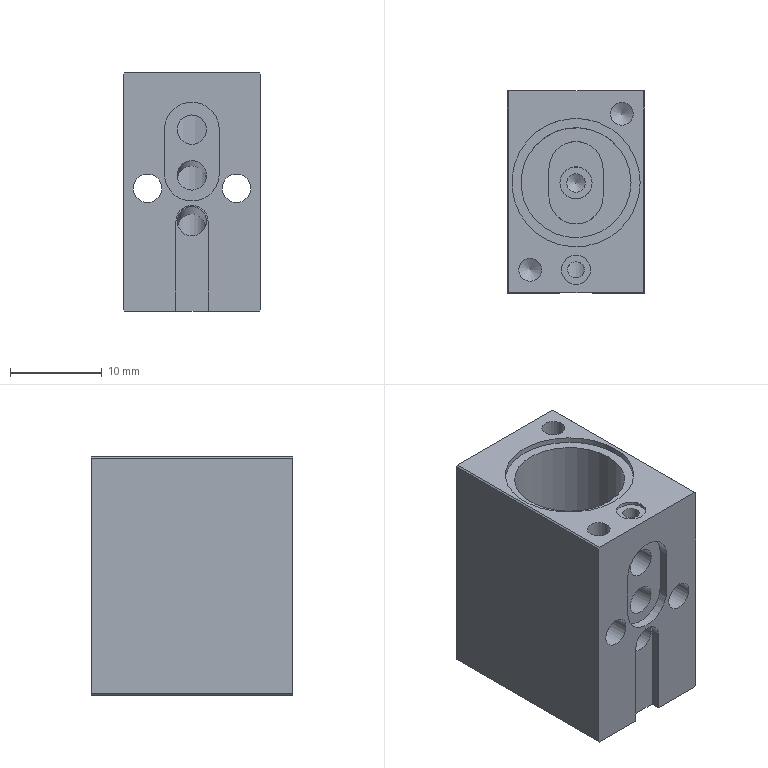NC program | NX | posted with a generic post | part box 15 x 22 x 26 mm
Whole program:
N10 G17 G21 G94 G90
(DRILLING_1 , TOOL : D3开粗)
N12 T14 M6
N14 G54
N16 G17 G0 G90 X-0.015 Y14.756 B0. C0. S3000 M3
N18 G43 Z3.431 H14
N20 G94 G81 G99 Z-0.569 F100. R3.431
N22 G80
(DRILLING_1_COPY , TOOL : D3开粗)
N24 G0 X-0.015 Y9.775
N26 G43 Z2.995 H14
N28 G81 Z-1.005 F100. R2.995
N30 G80
N32 M5
(DRILLING_1_COPY_1 , TOOL : D3点钻)
N34 T06 M6
N36 G54
N38 G17 G43 G0 G90 X-0.015 Y14.756 B0. C0. S3000 H6 M3
N40 Z3.431
N42 G94 G81 G99 Z-1.069 F200. R3.431
N44 G80
(DRILLING_1_COPY_COPY , TOOL : D3点钻)
N46 G0 X-0.015 Y9.775
N48 G43 Z2.995 H6
N50 G81 Z-1.505 F200. R2.995
N52 G80
N54 M5
(DRILLING_1_COPY_1_COPY , TOOL : D3.2钻头)
N56 T04 M6
N58 G54
N60 G17 G43 G0 G90 X-0.015 Y14.756 B0. C0. S3000 H4 M3
N62 Z3.431
N64 G94 G81 G99 Z-8.569 F200. R3.431
N66 G80
(DRILLING_1_COPY_COPY_COPY , TOOL : D3.2钻头)
N68 G0 X-0.015 Y9.775
N70 G43 Z2.995 H4
N72 G81 Z-12.005 F200. R2.995
N74 G80
N76 M5
(3_AXIS_DEBURRING , TOOL : R0.5)
N78 T18 M6
N80 G54
N82 G17 G43 G0 G90 X-0.959 Y9.797 B0. C0. S3000 H18 M3
N84 Z13.779
N86 Z0.214
N88 G94 G1 X-0.974 Y9.796 Z0.119 F243.
N90 X-1.013 Y9.793 Z0.028
N92 X-1.134 Y9.783 Z-0.131
N94 X-1.185 Y9.756 Z-0.19
N96 X-1.221 Y9.696 Z-0.245
N98 X-1.243 Y9.618 Z-0.292
N100 X-1.25 Y9.535 Z-0.325
N102 Y9.449 Z-0.352 F270.
N104 Y9.361 Z-0.38
N106 X-1.234 Y9.275 Z-0.408
N108 X-1.198 Y9.194 Z-0.416
N110 X-1.163 Y9.113 Z-0.424
N112 X-1.111 Y9.041 Z-0.431
N114 X-1.06 Y8.969 Z-0.438
N116 X-1.009 Y8.897 Z-0.445
N118 X-0.945 Y8.836 Z-0.451
N120 X-0.88 Y8.776 Z-0.457
N122 X-0.816 Y8.716 Z-0.463
N124 X-0.741 Y8.669 Z-0.467
N126 X-0.666 Y8.623 Z-0.472
N128 X-0.59 Y8.577 Z-0.476
N130 X-0.508 Y8.547 Z-0.479
N132 X-0.425 Y8.517 Z-0.483
N134 X-0.342 Y8.486 Z-0.486
N136 X-0.255 Y8.47 Z-0.484
N138 X-0.169 Y8.454 Z-0.483
N140 X-0.082 Y8.438 Z-0.482
N142 X-0.017 Y8.437 Z-0.478
N144 X0.047 Y8.435 Z-0.474
N146 X0.112 Y8.434 Z-0.47
N148 X0.176 Y8.432 Z-0.466
N150 X0.179
N152 X0.267 Y8.464 Z-0.471
N154 X0.352 Y8.495 Z-0.476
N156 X0.438 Y8.526 Z-0.482
N158 X0.517 Y8.564 Z-0.478
N160 X0.597 Y8.602 Z-0.474
N162 X0.676 Y8.641 Z-0.47
N164 X0.746 Y8.694 Z-0.465
N166 X0.816 Y8.748 Z-0.46
N168 X0.886 Y8.801 Z-0.454
N170 X0.944 Y8.868 Z-0.448
N172 X1.003 Y8.934 Z-0.441
N174 X1.061 Y9.001 Z-0.435
N176 X1.107 Y9.077 Z-0.425
N178 X1.152 Y9.153 Z-0.415
N180 X1.198 Y9.229 Z-0.405
N182 X1.222 Y9.314 Z-0.394
N184 Y9.404 Z-0.357
N186 Y9.49 Z-0.322
N188 X1.215 Y9.572 Z-0.281
N190 X1.194 Y9.649 Z-0.228
N192 X1.158 Y9.707 Z-0.168
N194 X1.107 Y9.734 Z-0.105
N196 X0.989 Y9.747 Z0.056
N198 X0.951 Y9.752 Z0.148
N200 X0.936 Y9.753 Z0.243
N202 X0.912 Y9.754 Z0.405
N204 X0.888 Y9.75 Z0.571
N206 X0.863 Y9.741 Z0.741
N208 X0.838 Y9.73 Z0.915
N210 X0.812 Y9.715 Z1.092
N212 X0.786 Y9.697 Z1.271
N214 X0.76 Y9.676 Z1.454
N216 X0.733 Y9.654 Z1.638
N218 X0.706 Y9.629 Z1.824
N220 X0.679 Y9.604 Z2.012
N222 X0.652 Y9.577 Z2.201
N224 X0.625 Y9.55 Z2.39
N226 X0.598 Y9.522 Z2.58
N228 X0.57 Y9.494 Z2.769
N230 X0.543 Y9.468 Z2.958
N232 X0.516 Y9.441 Z3.146
N234 X0.489 Y9.417 Z3.333
N236 X0.463 Y9.393 Z3.518
N238 X0.436 Y9.372 Z3.701
N240 X0.41 Y9.353 Z3.882
N242 X0.384 Y9.337 Z4.06
N244 X0.359 Y9.324 Z4.234
N246 X0.334 Y9.315 Z4.405
N248 X0.309 Y9.31 Z4.573
N250 X0.285 Y9.308 Z4.736
N252 X0.261 Y9.312 Z4.894
N254 X0.238 Y9.32 Z5.047
N256 X0.216 Y9.334 Z5.195
N258 X0.194 Y9.354 Z5.337
N260 X0.173 Y9.38 Z5.473
N262 X0.153 Y9.412 Z5.602
N264 X0.134 Y9.452 Z5.724
N266 X0.116 Y9.498 Z5.839
N268 X0.098 Y9.553 Z5.946
N270 X0.081 Y9.615 Z6.045
N272 X0.066 Y9.686 Z6.136
N274 X0.051 Y9.765 Z6.218
N276 X0.038 Y9.854 Z6.29
N278 X0.028 Y9.928 Z6.339
N280 X0.019 Y10.009 Z6.385
N282 X0.01 Y10.097 Z6.429
N284 X0.001 Y10.192 Z6.47
N286 X-0.008 Y10.294 Z6.509
N288 X-0.016 Y10.401 Z6.545
N290 X-0.024 Y10.514 Z6.578
N292 X-0.032 Y10.633 Z6.609
N294 X-0.04 Y10.756 Z6.637
N296 X-0.047 Y10.883 Z6.662
N298 X-0.054 Y11.014 Z6.685
N300 X-0.061 Y11.148 Z6.705
N302 X-0.067 Y11.285 Z6.723
N304 X-0.074 Y11.425 Z6.738
N306 X-0.079 Y11.567 Z6.75
N308 X-0.085 Y11.71 Z6.76
N310 X-0.09 Y11.855 Z6.767
N312 X-0.095 Y12. Z6.771
N314 X-0.099 Y12.145 Z6.773
N316 X-0.103 Y12.291 Z6.772
N318 X-0.107 Y12.435 Z6.768
N320 X-0.11 Y12.579 Z6.762
N322 X-0.113 Y12.721 Z6.753
N324 X-0.116 Y12.862 Z6.741
N326 X-0.118 Y13. Z6.727
N328 X-0.12 Y13.135 Z6.71
N330 X-0.121 Y13.267 Z6.69
N332 X-0.122 Y13.395 Z6.668
N334 Y13.519 Z6.642
N336 Y13.639 Z6.615
N338 Y13.754 Z6.584
N340 X-0.121 Y13.863 Z6.551
N342 X-0.119 Y13.966 Z6.515
N344 X-0.117 Y14.063 Z6.476
N346 X-0.115 Y14.154 Z6.434
N348 X-0.112 Y14.237 Z6.39
N350 X-0.108 Y14.312 Z6.343
N352 X-0.104 Y14.38 Z6.293
N354 X-0.098 Y14.458 Z6.222
N356 X-0.09 Y14.526 Z6.142
N358 X-0.081 Y14.584 Z6.054
N360 X-0.071 Y14.635 Z5.957
N362 X-0.06 Y14.676 Z5.853
N364 X-0.047 Y14.71 Z5.742
N366 X-0.033 Y14.736 Z5.623
N368 X-0.019 Y14.755 Z5.498
N370 X-0.003 Y14.767 Z5.366
N372 X0.014 Y14.772 Z5.229
N374 X0.031 Y14.771 Z5.086
N376 X0.05 Y14.765 Z4.938
N378 X0.069 Y14.754 Z4.785
N380 X0.088 Y14.737 Z4.627
N382 X0.109 Y14.717 Z4.466
N384 X0.13 Y14.692 Z4.3
N386 X0.151 Y14.663 Z4.132
N388 X0.173 Y14.631 Z3.96
N390 X0.196 Y14.597 Z3.786
N392 X0.219 Y14.559 Z3.609
N394 X0.242 Y14.52 Z3.431
N396 X0.265 Y14.479 Z3.25
N398 X0.289 Y14.437 Z3.069
N400 X0.312 Y14.393 Z2.887
N402 X0.336 Y14.35 Z2.704
N404 X0.36 Y14.306 Z2.521
N406 X0.383 Y14.262 Z2.339
N408 X0.407 Y14.219 Z2.157
N410 X0.43 Y14.177 Z1.976
N412 X0.454 Y14.136 Z1.796
N414 X0.477 Y14.098 Z1.618
N416 X0.499 Y14.061 Z1.443
N418 X0.522 Y14.028 Z1.269
N420 X0.544 Y13.997 Z1.098
N422 X0.565 Y13.969 Z0.931
N424 X0.586 Y13.946 Z0.767
N426 X0.606 Y13.926 Z0.606
N428 X0.625 Y13.912 Z0.45
N430 X0.638 Y13.904 Z0.354 F243.
N432 X0.669 Y13.883 Z0.262
N434 X0.769 Y13.819 Z0.101
N436 X0.825 Y13.812 Z0.052
N438 X0.896 Y13.839 Z0.019
N440 X0.969 Y13.888 Z0.001
N442 X1.03 Y13.945 Z-0.001
N444 X1.062 Y13.981 Z0.003 F270.
N446 X1.105 Y14.058 Z0.01
N448 X1.149 Y14.135 Z0.017
N450 X1.193 Y14.213 Z0.025
N452 X1.22 Y14.297 Z0.033
N454 X1.247 Y14.382 Z0.041
N456 X1.275 Y14.466 Z0.049
N458 X1.284 Y14.555 Z0.057
N460 X1.292 Y14.643 Z0.064
N462 X1.301 Y14.732 Z0.072
N464 X1.294 Y14.82 Z0.081
N466 X1.286 Y14.909 Z0.09
N468 X1.279 Y14.997 Z0.1
N470 X1.253 Y15.083 Z0.108
N472 X1.227 Y15.168 Z0.116
N474 X1.201 Y15.254 Z0.124
N476 X1.158 Y15.332 Z0.132
N478 X1.115 Y15.41 Z0.139
N480 X1.072 Y15.489 Z0.147
N482 X1.014 Y15.557 Z0.154
N484 X0.957 Y15.625 Z0.16
N486 X0.899 Y15.694 Z0.167
N488 X0.828 Y15.749 Z0.172
N490 X0.758 Y15.804 Z0.177
N492 X0.687 Y15.859 Z0.182
N494 X0.607 Y15.899 Z0.186
N496 X0.526 Y15.939 Z0.19
N498 X0.446 Y15.978 Z0.194
N500 X0.361 Y16.002 Z0.197
N502 X0.276 Y16.026 Z0.201
N504 X0.191 Y16.05 Z0.205
N506 X0.112 Y16.058 Z0.21
N508 X0.033 Y16.066 Z0.215
N510 X-0.046 Y16.074 Z0.221
N512 X-0.125 Y16.082 Z0.226
N514 X-0.207 Y16.06 Z0.217
N516 X-0.289 Y16.037 Z0.208
N518 X-0.37 Y16.014 Z0.198
N520 X-0.49 Y15.967 Z0.193
N522 X-0.609 Y15.921 Z0.188
N524 X-0.664 Y15.886 Z0.185
N526 X-0.718 Y15.851 Z0.182
N528 X-0.773 Y15.817 Z0.178
N530 X-0.828 Y15.782 Z0.175
N532 X-0.892 Y15.72 Z0.169
N534 X-0.957 Y15.658 Z0.163
N536 X-1.021 Y15.596 Z0.157
N538 X-1.072 Y15.522 Z0.15
N540 X-1.122 Y15.448 Z0.143
N542 X-1.173 Y15.374 Z0.136
N544 X-1.208 Y15.292 Z0.128
N546 X-1.242 Y15.21 Z0.12
N548 X-1.277 Y15.127 Z0.112
N550 X-1.294 Y15.04 Z0.104
N552 X-1.311 Y14.952 Z0.095
N554 X-1.328 Y14.865 Z0.087
N556 X-1.327 Y14.776 Z0.078
N558 X-1.326 Y14.687 Z0.07
N560 X-1.325 Y14.598 Z0.061
N562 X-1.309 Y14.51 Z0.055
N564 X-1.292 Y14.423 Z0.048
N566 X-1.276 Y14.335 Z0.042
N568 X-1.24 Y14.254 Z0.034
N570 X-1.203 Y14.172 Z0.025
N572 X-1.167 Y14.091 Z0.017
N574 X-1.116 Y14.019 Z0.01
N576 X-1.064 Y13.946 Z0.003
N578 X-1.013 Y13.874 Z-0.004
N580 X-0.952 Y13.807
N582 X-0.892 Y13.741
N584 X-0.831 Y13.675 Z-0.005
N586 X-0.771 Y13.646 Z-0.014
N588 X-0.711 Y13.616 Z-0.023
N590 X-0.651 Y13.587 Z-0.032
N592 X-0.59 Y13.558 Z-0.041
N594 X-0.508 Y13.525
N596 X-0.426 Y13.492 Z-0.042
N598 X-0.344 Y13.459
N600 X-0.257 Y13.446 Z-0.044
N602 X-0.169 Y13.434 Z-0.046
N604 X-0.082 Y13.421 Z-0.048
N606 X-0.016 Y13.419 Z-0.043
N608 X0.05 Y13.418 Z-0.039
N610 X0.115 Y13.416 Z-0.035
N612 X0.181 Y13.414 Z-0.03
N614 X0.184
N616 X0.249 Y13.438 Z-0.034
N618 X0.312 Y13.461 Z-0.038
N620 X0.375 Y13.484 Z-0.042
N622 X0.438 Y13.507 Z-0.046
N624 X0.517 Y13.545 Z-0.042
N626 X0.597 Y13.583 Z-0.038
N628 X0.676 Y13.622 Z-0.034
N630 X0.746 Y13.675 Z-0.029
N632 X0.816 Y13.729 Z-0.024
N634 X0.886 Y13.782 Z-0.018
N636 X0.945 Y13.848 Z-0.011
N638 X1.003 Y13.915 Z-0.004
N640 X1.03 Y13.945 Z-0.001
N642 X1.076 Y14.009 Z0.014
N644 X1.11 Y14.083 Z0.046
N646 X1.121 Y14.149 Z0.089
N648 X1.099 Y14.193 Z0.14
N650 X0.999 Y14.257 Z0.302
N652 X0.967 Y14.278 Z0.394
N654 X0.955 Y14.285 Z0.489
N656 G0 Z13.779
N658 M5
N660 M2